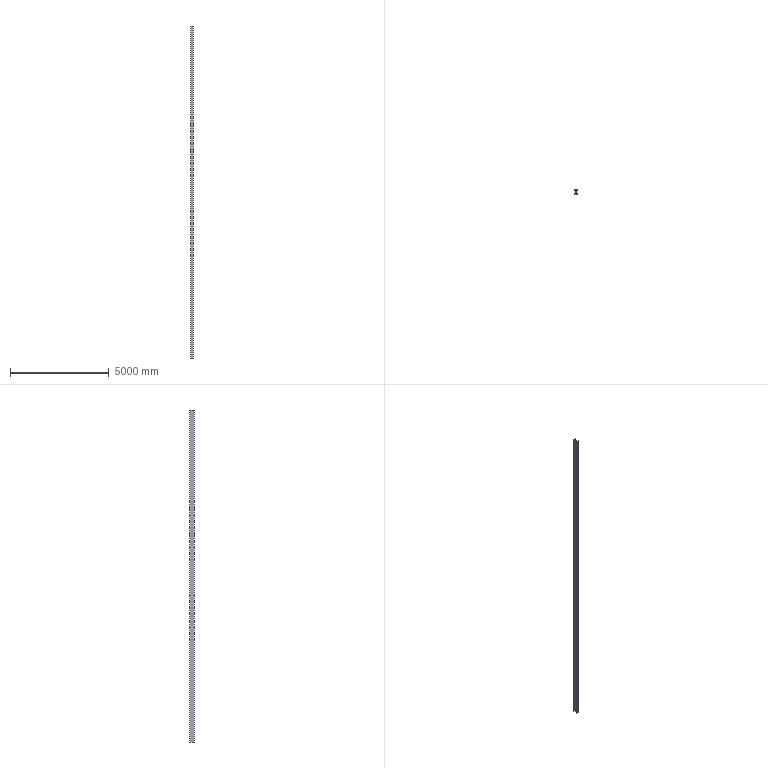Part | SolidWorks | features Extrusion 1 | 1 solid | 18 faces | box 125 x 250 x 16840 mm | volume 62256437 mm3 | plane 14 | cylinder 4 | commonest cylinder face diameters 16 x4
STEP:
#1=CARTESIAN_POINT('',(-62.5,9.,0.));
#2=VERTEX_POINT('',#1);
#3=CARTESIAN_POINT('',(-62.5,0.,0.));
#4=VERTEX_POINT('',#3);
#5=CARTESIAN_POINT('',(-62.5,0.,0.));
#6=DIRECTION('',(0.,-1.,0.));
#7=VECTOR('',#6,1000.);
#8=LINE('',#5,#7);
#9=EDGE_CURVE('',#2,#4,#8,.T.);
#10=ORIENTED_EDGE('',*,*,#9,.T.);
#11=CARTESIAN_POINT('',(-62.5,0.,16840.));
#12=VERTEX_POINT('',#11);
#13=CARTESIAN_POINT('',(-62.5,0.,16840.));
#14=DIRECTION('',(0.,0.,-1.));
#15=VECTOR('',#14,1000.);
#16=LINE('',#13,#15);
#17=EDGE_CURVE('',#12,#4,#16,.T.);
#18=ORIENTED_EDGE('',*,*,#17,.F.);
#19=CARTESIAN_POINT('',(-62.5,9.,16840.));
#20=VERTEX_POINT('',#19);
#21=CARTESIAN_POINT('',(-62.5,0.,16840.));
#22=DIRECTION('',(0.,-1.,0.));
#23=VECTOR('',#22,1000.);
#24=LINE('',#21,#23);
#25=EDGE_CURVE('',#20,#12,#24,.T.);
#26=ORIENTED_EDGE('',*,*,#25,.F.);
#27=CARTESIAN_POINT('',(-62.5,9.,16840.));
#28=DIRECTION('',(0.,0.,-1.));
#29=VECTOR('',#28,1000.);
#30=LINE('',#27,#29);
#31=EDGE_CURVE('',#20,#2,#30,.T.);
#32=ORIENTED_EDGE('',*,*,#31,.T.);
#33=EDGE_LOOP('',(#10,#18,#26,#32));
#34=FACE_OUTER_BOUND('',#33,.T.);
#35=CARTESIAN_POINT('',(-62.5,0.,16840.));
#36=DIRECTION('',(1.,0.,0.));
#37=DIRECTION('',(0.,0.,-1.));
#38=AXIS2_PLACEMENT_3D('',#35,#36,#37);
#39=PLANE('',#38);
#40=ADVANCED_FACE('',(#34),#39,.F.);
#41=CARTESIAN_POINT('',(62.5,0.,0.));
#42=VERTEX_POINT('',#41);
#43=CARTESIAN_POINT('',(62.5,0.,0.));
#44=DIRECTION('',(1.,0.,0.));
#45=VECTOR('',#44,1000.);
#46=LINE('',#43,#45);
#47=EDGE_CURVE('',#4,#42,#46,.T.);
#48=ORIENTED_EDGE('',*,*,#47,.T.);
#49=CARTESIAN_POINT('',(62.5,0.,16840.));
#50=VERTEX_POINT('',#49);
#51=CARTESIAN_POINT('',(62.5,0.,16840.));
#52=DIRECTION('',(0.,0.,-1.));
#53=VECTOR('',#52,1000.);
#54=LINE('',#51,#53);
#55=EDGE_CURVE('',#50,#42,#54,.T.);
#56=ORIENTED_EDGE('',*,*,#55,.F.);
#57=CARTESIAN_POINT('',(62.5,0.,16840.));
#58=DIRECTION('',(1.,0.,0.));
#59=VECTOR('',#58,1000.);
#60=LINE('',#57,#59);
#61=EDGE_CURVE('',#12,#50,#60,.T.);
#62=ORIENTED_EDGE('',*,*,#61,.F.);
#63=ORIENTED_EDGE('',*,*,#17,.T.);
#64=EDGE_LOOP('',(#48,#56,#62,#63));
#65=FACE_OUTER_BOUND('',#64,.T.);
#66=CARTESIAN_POINT('',(62.5,0.,16840.));
#67=DIRECTION('',(0.,1.,0.));
#68=DIRECTION('',(0.,0.,1.));
#69=AXIS2_PLACEMENT_3D('',#66,#67,#68);
#70=PLANE('',#69);
#71=ADVANCED_FACE('',(#65),#70,.F.);
#72=CARTESIAN_POINT('',(62.5,9.,0.));
#73=VERTEX_POINT('',#72);
#74=CARTESIAN_POINT('',(62.5,0.,0.));
#75=DIRECTION('',(0.,1.,0.));
#76=VECTOR('',#75,1000.);
#77=LINE('',#74,#76);
#78=EDGE_CURVE('',#42,#73,#77,.T.);
#79=ORIENTED_EDGE('',*,*,#78,.T.);
#80=CARTESIAN_POINT('',(62.5,9.,16840.));
#81=VERTEX_POINT('',#80);
#82=CARTESIAN_POINT('',(62.5,9.,16840.));
#83=DIRECTION('',(0.,0.,-1.));
#84=VECTOR('',#83,1000.);
#85=LINE('',#82,#84);
#86=EDGE_CURVE('',#81,#73,#85,.T.);
#87=ORIENTED_EDGE('',*,*,#86,.F.);
#88=CARTESIAN_POINT('',(62.5,0.,16840.));
#89=DIRECTION('',(0.,1.,0.));
#90=VECTOR('',#89,1000.);
#91=LINE('',#88,#90);
#92=EDGE_CURVE('',#50,#81,#91,.T.);
#93=ORIENTED_EDGE('',*,*,#92,.F.);
#94=ORIENTED_EDGE('',*,*,#55,.T.);
#95=EDGE_LOOP('',(#79,#87,#93,#94));
#96=FACE_OUTER_BOUND('',#95,.T.);
#97=CARTESIAN_POINT('',(62.5,0.,16840.));
#98=DIRECTION('',(-1.,0.,0.));
#99=DIRECTION('',(0.,0.,1.));
#100=AXIS2_PLACEMENT_3D('',#97,#98,#99);
#101=PLANE('',#100);
#102=ADVANCED_FACE('',(#96),#101,.F.);
#103=CARTESIAN_POINT('',(11.,9.,0.));
#104=VERTEX_POINT('',#103);
#105=CARTESIAN_POINT('',(62.5,9.,0.));
#106=DIRECTION('',(-1.,0.,0.));
#107=VECTOR('',#106,1000.);
#108=LINE('',#105,#107);
#109=EDGE_CURVE('',#73,#104,#108,.T.);
#110=ORIENTED_EDGE('',*,*,#109,.T.);
#111=CARTESIAN_POINT('',(11.,9.,16840.));
#112=VERTEX_POINT('',#111);
#113=CARTESIAN_POINT('',(11.,9.,16840.));
#114=DIRECTION('',(0.,0.,-1.));
#115=VECTOR('',#114,1000.);
#116=LINE('',#113,#115);
#117=EDGE_CURVE('',#112,#104,#116,.T.);
#118=ORIENTED_EDGE('',*,*,#117,.F.);
#119=CARTESIAN_POINT('',(62.5,9.,16840.));
#120=DIRECTION('',(-1.,0.,0.));
#121=VECTOR('',#120,1000.);
#122=LINE('',#119,#121);
#123=EDGE_CURVE('',#81,#112,#122,.T.);
#124=ORIENTED_EDGE('',*,*,#123,.F.);
#125=ORIENTED_EDGE('',*,*,#86,.T.);
#126=EDGE_LOOP('',(#110,#118,#124,#125));
#127=FACE_OUTER_BOUND('',#126,.T.);
#128=CARTESIAN_POINT('',(62.5,9.,16840.));
#129=DIRECTION('',(0.,-1.,0.));
#130=DIRECTION('',(0.,0.,-1.));
#131=AXIS2_PLACEMENT_3D('',#128,#129,#130);
#132=PLANE('',#131);
#133=ADVANCED_FACE('',(#127),#132,.F.);
#134=CARTESIAN_POINT('',(3.,17.,0.));
#135=VERTEX_POINT('',#134);
#136=CARTESIAN_POINT('',(11.,17.,0.));
#137=DIRECTION('',(0.,0.,-1.));
#138=DIRECTION('',(-1.,0.,0.));
#139=AXIS2_PLACEMENT_3D('',#136,#137,#138);
#140=CIRCLE('',#139,8.);
#141=EDGE_CURVE('',#104,#135,#140,.T.);
#142=ORIENTED_EDGE('',*,*,#141,.T.);
#143=CARTESIAN_POINT('',(3.,17.,16840.));
#144=VERTEX_POINT('',#143);
#145=CARTESIAN_POINT('',(3.,17.,16840.));
#146=DIRECTION('',(0.,0.,-1.));
#147=VECTOR('',#146,1000.);
#148=LINE('',#145,#147);
#149=EDGE_CURVE('',#144,#135,#148,.T.);
#150=ORIENTED_EDGE('',*,*,#149,.F.);
#151=CARTESIAN_POINT('',(11.,17.,16840.));
#152=DIRECTION('',(0.,0.,-1.));
#153=DIRECTION('',(-1.,0.,0.));
#154=AXIS2_PLACEMENT_3D('',#151,#152,#153);
#155=CIRCLE('',#154,8.);
#156=EDGE_CURVE('',#112,#144,#155,.T.);
#157=ORIENTED_EDGE('',*,*,#156,.F.);
#158=ORIENTED_EDGE('',*,*,#117,.T.);
#159=EDGE_LOOP('',(#142,#150,#157,#158));
#160=FACE_OUTER_BOUND('',#159,.T.);
#161=CARTESIAN_POINT('',(11.,17.,16840.));
#162=DIRECTION('',(0.,0.,-1.));
#163=DIRECTION('',(-1.,0.,0.));
#164=AXIS2_PLACEMENT_3D('',#161,#162,#163);
#165=CYLINDRICAL_SURFACE('',#164,8.);
#166=ADVANCED_FACE('',(#160),#165,.F.);
#167=CARTESIAN_POINT('',(3.,233.,0.));
#168=VERTEX_POINT('',#167);
#169=CARTESIAN_POINT('',(3.,17.,0.));
#170=DIRECTION('',(0.,1.,0.));
#171=VECTOR('',#170,1000.);
#172=LINE('',#169,#171);
#173=EDGE_CURVE('',#135,#168,#172,.T.);
#174=ORIENTED_EDGE('',*,*,#173,.T.);
#175=CARTESIAN_POINT('',(3.,233.,16840.));
#176=VERTEX_POINT('',#175);
#177=CARTESIAN_POINT('',(3.,233.,16840.));
#178=DIRECTION('',(0.,0.,-1.));
#179=VECTOR('',#178,1000.);
#180=LINE('',#177,#179);
#181=EDGE_CURVE('',#176,#168,#180,.T.);
#182=ORIENTED_EDGE('',*,*,#181,.F.);
#183=CARTESIAN_POINT('',(3.,17.,16840.));
#184=DIRECTION('',(0.,1.,0.));
#185=VECTOR('',#184,1000.);
#186=LINE('',#183,#185);
#187=EDGE_CURVE('',#144,#176,#186,.T.);
#188=ORIENTED_EDGE('',*,*,#187,.F.);
#189=ORIENTED_EDGE('',*,*,#149,.T.);
#190=EDGE_LOOP('',(#174,#182,#188,#189));
#191=FACE_OUTER_BOUND('',#190,.T.);
#192=CARTESIAN_POINT('',(3.,17.,16840.));
#193=DIRECTION('',(-1.,0.,0.));
#194=DIRECTION('',(0.,-1.,0.));
#195=AXIS2_PLACEMENT_3D('',#192,#193,#194);
#196=PLANE('',#195);
#197=ADVANCED_FACE('',(#191),#196,.F.);
#198=CARTESIAN_POINT('',(11.,241.,0.));
#199=VERTEX_POINT('',#198);
#200=CARTESIAN_POINT('',(11.,233.,0.));
#201=DIRECTION('',(0.,0.,-1.));
#202=DIRECTION('',(-1.,0.,0.));
#203=AXIS2_PLACEMENT_3D('',#200,#201,#202);
#204=CIRCLE('',#203,8.);
#205=EDGE_CURVE('',#168,#199,#204,.T.);
#206=ORIENTED_EDGE('',*,*,#205,.T.);
#207=CARTESIAN_POINT('',(11.,241.,16840.));
#208=VERTEX_POINT('',#207);
#209=CARTESIAN_POINT('',(11.,241.,16840.));
#210=DIRECTION('',(0.,0.,-1.));
#211=VECTOR('',#210,1000.);
#212=LINE('',#209,#211);
#213=EDGE_CURVE('',#208,#199,#212,.T.);
#214=ORIENTED_EDGE('',*,*,#213,.F.);
#215=CARTESIAN_POINT('',(11.,233.,16840.));
#216=DIRECTION('',(0.,0.,-1.));
#217=DIRECTION('',(-1.,0.,0.));
#218=AXIS2_PLACEMENT_3D('',#215,#216,#217);
#219=CIRCLE('',#218,8.);
#220=EDGE_CURVE('',#176,#208,#219,.T.);
#221=ORIENTED_EDGE('',*,*,#220,.F.);
#222=ORIENTED_EDGE('',*,*,#181,.T.);
#223=EDGE_LOOP('',(#206,#214,#221,#222));
#224=FACE_OUTER_BOUND('',#223,.T.);
#225=CARTESIAN_POINT('',(11.,233.,16840.));
#226=DIRECTION('',(0.,0.,-1.));
#227=DIRECTION('',(-1.,0.,0.));
#228=AXIS2_PLACEMENT_3D('',#225,#226,#227);
#229=CYLINDRICAL_SURFACE('',#228,8.);
#230=ADVANCED_FACE('',(#224),#229,.F.);
#231=CARTESIAN_POINT('',(62.5,241.,0.));
#232=VERTEX_POINT('',#231);
#233=CARTESIAN_POINT('',(11.,241.,0.));
#234=DIRECTION('',(1.,0.,0.));
#235=VECTOR('',#234,1000.);
#236=LINE('',#233,#235);
#237=EDGE_CURVE('',#199,#232,#236,.T.);
#238=ORIENTED_EDGE('',*,*,#237,.T.);
#239=CARTESIAN_POINT('',(62.5,241.,16840.));
#240=VERTEX_POINT('',#239);
#241=CARTESIAN_POINT('',(62.5,241.,16840.));
#242=DIRECTION('',(0.,0.,-1.));
#243=VECTOR('',#242,1000.);
#244=LINE('',#241,#243);
#245=EDGE_CURVE('',#240,#232,#244,.T.);
#246=ORIENTED_EDGE('',*,*,#245,.F.);
#247=CARTESIAN_POINT('',(11.,241.,16840.));
#248=DIRECTION('',(1.,0.,0.));
#249=VECTOR('',#248,1000.);
#250=LINE('',#247,#249);
#251=EDGE_CURVE('',#208,#240,#250,.T.);
#252=ORIENTED_EDGE('',*,*,#251,.F.);
#253=ORIENTED_EDGE('',*,*,#213,.T.);
#254=EDGE_LOOP('',(#238,#246,#252,#253));
#255=FACE_OUTER_BOUND('',#254,.T.);
#256=CARTESIAN_POINT('',(11.,241.,16840.));
#257=DIRECTION('',(0.,1.,0.));
#258=DIRECTION('',(0.,0.,1.));
#259=AXIS2_PLACEMENT_3D('',#256,#257,#258);
#260=PLANE('',#259);
#261=ADVANCED_FACE('',(#255),#260,.F.);
#262=CARTESIAN_POINT('',(62.5,250.,0.));
#263=VERTEX_POINT('',#262);
#264=CARTESIAN_POINT('',(62.5,241.,0.));
#265=DIRECTION('',(0.,1.,0.));
#266=VECTOR('',#265,1000.);
#267=LINE('',#264,#266);
#268=EDGE_CURVE('',#232,#263,#267,.T.);
#269=ORIENTED_EDGE('',*,*,#268,.T.);
#270=CARTESIAN_POINT('',(62.5,250.,16840.));
#271=VERTEX_POINT('',#270);
#272=CARTESIAN_POINT('',(62.5,250.,16840.));
#273=DIRECTION('',(0.,0.,-1.));
#274=VECTOR('',#273,1000.);
#275=LINE('',#272,#274);
#276=EDGE_CURVE('',#271,#263,#275,.T.);
#277=ORIENTED_EDGE('',*,*,#276,.F.);
#278=CARTESIAN_POINT('',(62.5,241.,16840.));
#279=DIRECTION('',(0.,1.,0.));
#280=VECTOR('',#279,1000.);
#281=LINE('',#278,#280);
#282=EDGE_CURVE('',#240,#271,#281,.T.);
#283=ORIENTED_EDGE('',*,*,#282,.F.);
#284=ORIENTED_EDGE('',*,*,#245,.T.);
#285=EDGE_LOOP('',(#269,#277,#283,#284));
#286=FACE_OUTER_BOUND('',#285,.T.);
#287=CARTESIAN_POINT('',(62.5,241.,16840.));
#288=DIRECTION('',(-1.,0.,0.));
#289=DIRECTION('',(0.,0.,1.));
#290=AXIS2_PLACEMENT_3D('',#287,#288,#289);
#291=PLANE('',#290);
#292=ADVANCED_FACE('',(#286),#291,.F.);
#293=CARTESIAN_POINT('',(-62.5,250.,0.));
#294=VERTEX_POINT('',#293);
#295=CARTESIAN_POINT('',(-62.5,250.,0.));
#296=DIRECTION('',(-1.,0.,0.));
#297=VECTOR('',#296,1000.);
#298=LINE('',#295,#297);
#299=EDGE_CURVE('',#263,#294,#298,.T.);
#300=ORIENTED_EDGE('',*,*,#299,.T.);
#301=CARTESIAN_POINT('',(-62.5,250.,16840.));
#302=VERTEX_POINT('',#301);
#303=CARTESIAN_POINT('',(-62.5,250.,16840.));
#304=DIRECTION('',(0.,0.,-1.));
#305=VECTOR('',#304,1000.);
#306=LINE('',#303,#305);
#307=EDGE_CURVE('',#302,#294,#306,.T.);
#308=ORIENTED_EDGE('',*,*,#307,.F.);
#309=CARTESIAN_POINT('',(-62.5,250.,16840.));
#310=DIRECTION('',(-1.,0.,0.));
#311=VECTOR('',#310,1000.);
#312=LINE('',#309,#311);
#313=EDGE_CURVE('',#271,#302,#312,.T.);
#314=ORIENTED_EDGE('',*,*,#313,.F.);
#315=ORIENTED_EDGE('',*,*,#276,.T.);
#316=EDGE_LOOP('',(#300,#308,#314,#315));
#317=FACE_OUTER_BOUND('',#316,.T.);
#318=CARTESIAN_POINT('',(-62.5,250.,16840.));
#319=DIRECTION('',(0.,-1.,0.));
#320=DIRECTION('',(1.,0.,0.));
#321=AXIS2_PLACEMENT_3D('',#318,#319,#320);
#322=PLANE('',#321);
#323=ADVANCED_FACE('',(#317),#322,.F.);
#324=CARTESIAN_POINT('',(-62.5,241.,0.));
#325=VERTEX_POINT('',#324);
#326=CARTESIAN_POINT('',(-62.5,241.,0.));
#327=DIRECTION('',(0.,-1.,0.));
#328=VECTOR('',#327,1000.);
#329=LINE('',#326,#328);
#330=EDGE_CURVE('',#294,#325,#329,.T.);
#331=ORIENTED_EDGE('',*,*,#330,.T.);
#332=CARTESIAN_POINT('',(-62.5,241.,16840.));
#333=VERTEX_POINT('',#332);
#334=CARTESIAN_POINT('',(-62.5,241.,16840.));
#335=DIRECTION('',(0.,0.,-1.));
#336=VECTOR('',#335,1000.);
#337=LINE('',#334,#336);
#338=EDGE_CURVE('',#333,#325,#337,.T.);
#339=ORIENTED_EDGE('',*,*,#338,.F.);
#340=CARTESIAN_POINT('',(-62.5,241.,16840.));
#341=DIRECTION('',(0.,-1.,0.));
#342=VECTOR('',#341,1000.);
#343=LINE('',#340,#342);
#344=EDGE_CURVE('',#302,#333,#343,.T.);
#345=ORIENTED_EDGE('',*,*,#344,.F.);
#346=ORIENTED_EDGE('',*,*,#307,.T.);
#347=EDGE_LOOP('',(#331,#339,#345,#346));
#348=FACE_OUTER_BOUND('',#347,.T.);
#349=CARTESIAN_POINT('',(-62.5,241.,16840.));
#350=DIRECTION('',(1.,0.,0.));
#351=DIRECTION('',(0.,0.,-1.));
#352=AXIS2_PLACEMENT_3D('',#349,#350,#351);
#353=PLANE('',#352);
#354=ADVANCED_FACE('',(#348),#353,.F.);
#355=CARTESIAN_POINT('',(-11.,241.,0.));
#356=VERTEX_POINT('',#355);
#357=CARTESIAN_POINT('',(-11.,241.,0.));
#358=DIRECTION('',(1.,0.,0.));
#359=VECTOR('',#358,1000.);
#360=LINE('',#357,#359);
#361=EDGE_CURVE('',#325,#356,#360,.T.);
#362=ORIENTED_EDGE('',*,*,#361,.T.);
#363=CARTESIAN_POINT('',(-11.,241.,16840.));
#364=VERTEX_POINT('',#363);
#365=CARTESIAN_POINT('',(-11.,241.,16840.));
#366=DIRECTION('',(0.,0.,-1.));
#367=VECTOR('',#366,1000.);
#368=LINE('',#365,#367);
#369=EDGE_CURVE('',#364,#356,#368,.T.);
#370=ORIENTED_EDGE('',*,*,#369,.F.);
#371=CARTESIAN_POINT('',(-11.,241.,16840.));
#372=DIRECTION('',(1.,0.,0.));
#373=VECTOR('',#372,1000.);
#374=LINE('',#371,#373);
#375=EDGE_CURVE('',#333,#364,#374,.T.);
#376=ORIENTED_EDGE('',*,*,#375,.F.);
#377=ORIENTED_EDGE('',*,*,#338,.T.);
#378=EDGE_LOOP('',(#362,#370,#376,#377));
#379=FACE_OUTER_BOUND('',#378,.T.);
#380=CARTESIAN_POINT('',(-11.,241.,16840.));
#381=DIRECTION('',(0.,1.,0.));
#382=DIRECTION('',(0.,0.,1.));
#383=AXIS2_PLACEMENT_3D('',#380,#381,#382);
#384=PLANE('',#383);
#385=ADVANCED_FACE('',(#379),#384,.F.);
#386=CARTESIAN_POINT('',(-3.,233.,0.));
#387=VERTEX_POINT('',#386);
#388=CARTESIAN_POINT('',(-11.,233.,0.));
#389=DIRECTION('',(0.,0.,-1.));
#390=DIRECTION('',(1.,0.,0.));
#391=AXIS2_PLACEMENT_3D('',#388,#389,#390);
#392=CIRCLE('',#391,8.);
#393=EDGE_CURVE('',#356,#387,#392,.T.);
#394=ORIENTED_EDGE('',*,*,#393,.T.);
#395=CARTESIAN_POINT('',(-3.,233.,16840.));
#396=VERTEX_POINT('',#395);
#397=CARTESIAN_POINT('',(-3.,233.,16840.));
#398=DIRECTION('',(0.,0.,-1.));
#399=VECTOR('',#398,1000.);
#400=LINE('',#397,#399);
#401=EDGE_CURVE('',#396,#387,#400,.T.);
#402=ORIENTED_EDGE('',*,*,#401,.F.);
#403=CARTESIAN_POINT('',(-11.,233.,16840.));
#404=DIRECTION('',(0.,0.,-1.));
#405=DIRECTION('',(1.,0.,0.));
#406=AXIS2_PLACEMENT_3D('',#403,#404,#405);
#407=CIRCLE('',#406,8.);
#408=EDGE_CURVE('',#364,#396,#407,.T.);
#409=ORIENTED_EDGE('',*,*,#408,.F.);
#410=ORIENTED_EDGE('',*,*,#369,.T.);
#411=EDGE_LOOP('',(#394,#402,#409,#410));
#412=FACE_OUTER_BOUND('',#411,.T.);
#413=CARTESIAN_POINT('',(-11.,233.,16840.));
#414=DIRECTION('',(0.,0.,-1.));
#415=DIRECTION('',(-1.,0.,0.));
#416=AXIS2_PLACEMENT_3D('',#413,#414,#415);
#417=CYLINDRICAL_SURFACE('',#416,8.);
#418=ADVANCED_FACE('',(#412),#417,.F.);
#419=CARTESIAN_POINT('',(-3.,17.,0.));
#420=VERTEX_POINT('',#419);
#421=CARTESIAN_POINT('',(-3.,17.,0.));
#422=DIRECTION('',(0.,-1.,0.));
#423=VECTOR('',#422,1000.);
#424=LINE('',#421,#423);
#425=EDGE_CURVE('',#387,#420,#424,.T.);
#426=ORIENTED_EDGE('',*,*,#425,.T.);
#427=CARTESIAN_POINT('',(-3.,17.,16840.));
#428=VERTEX_POINT('',#427);
#429=CARTESIAN_POINT('',(-3.,17.,16840.));
#430=DIRECTION('',(0.,0.,-1.));
#431=VECTOR('',#430,1000.);
#432=LINE('',#429,#431);
#433=EDGE_CURVE('',#428,#420,#432,.T.);
#434=ORIENTED_EDGE('',*,*,#433,.F.);
#435=CARTESIAN_POINT('',(-3.,17.,16840.));
#436=DIRECTION('',(0.,-1.,0.));
#437=VECTOR('',#436,1000.);
#438=LINE('',#435,#437);
#439=EDGE_CURVE('',#396,#428,#438,.T.);
#440=ORIENTED_EDGE('',*,*,#439,.F.);
#441=ORIENTED_EDGE('',*,*,#401,.T.);
#442=EDGE_LOOP('',(#426,#434,#440,#441));
#443=FACE_OUTER_BOUND('',#442,.T.);
#444=CARTESIAN_POINT('',(-3.,17.,16840.));
#445=DIRECTION('',(1.,0.,0.));
#446=DIRECTION('',(0.,1.,0.));
#447=AXIS2_PLACEMENT_3D('',#444,#445,#446);
#448=PLANE('',#447);
#449=ADVANCED_FACE('',(#443),#448,.F.);
#450=CARTESIAN_POINT('',(-11.,9.,0.));
#451=VERTEX_POINT('',#450);
#452=CARTESIAN_POINT('',(-11.,17.,0.));
#453=DIRECTION('',(0.,0.,-1.));
#454=DIRECTION('',(-1.,0.,0.));
#455=AXIS2_PLACEMENT_3D('',#452,#453,#454);
#456=CIRCLE('',#455,8.);
#457=EDGE_CURVE('',#420,#451,#456,.T.);
#458=ORIENTED_EDGE('',*,*,#457,.T.);
#459=CARTESIAN_POINT('',(-11.,9.,16840.));
#460=VERTEX_POINT('',#459);
#461=CARTESIAN_POINT('',(-11.,9.,16840.));
#462=DIRECTION('',(0.,0.,-1.));
#463=VECTOR('',#462,1000.);
#464=LINE('',#461,#463);
#465=EDGE_CURVE('',#460,#451,#464,.T.);
#466=ORIENTED_EDGE('',*,*,#465,.F.);
#467=CARTESIAN_POINT('',(-11.,17.,16840.));
#468=DIRECTION('',(0.,0.,-1.));
#469=DIRECTION('',(-1.,0.,0.));
#470=AXIS2_PLACEMENT_3D('',#467,#468,#469);
#471=CIRCLE('',#470,8.);
#472=EDGE_CURVE('',#428,#460,#471,.T.);
#473=ORIENTED_EDGE('',*,*,#472,.F.);
#474=ORIENTED_EDGE('',*,*,#433,.T.);
#475=EDGE_LOOP('',(#458,#466,#473,#474));
#476=FACE_OUTER_BOUND('',#475,.T.);
#477=CARTESIAN_POINT('',(-11.,17.,16840.));
#478=DIRECTION('',(0.,0.,-1.));
#479=DIRECTION('',(-1.,0.,0.));
#480=AXIS2_PLACEMENT_3D('',#477,#478,#479);
#481=CYLINDRICAL_SURFACE('',#480,8.);
#482=ADVANCED_FACE('',(#476),#481,.F.);
#483=CARTESIAN_POINT('',(-62.5,9.,0.));
#484=DIRECTION('',(-1.,0.,0.));
#485=VECTOR('',#484,1000.);
#486=LINE('',#483,#485);
#487=EDGE_CURVE('',#451,#2,#486,.T.);
#488=ORIENTED_EDGE('',*,*,#487,.T.);
#489=ORIENTED_EDGE('',*,*,#31,.F.);
#490=CARTESIAN_POINT('',(-62.5,9.,16840.));
#491=DIRECTION('',(-1.,0.,0.));
#492=VECTOR('',#491,1000.);
#493=LINE('',#490,#492);
#494=EDGE_CURVE('',#460,#20,#493,.T.);
#495=ORIENTED_EDGE('',*,*,#494,.F.);
#496=ORIENTED_EDGE('',*,*,#465,.T.);
#497=EDGE_LOOP('',(#488,#489,#495,#496));
#498=FACE_OUTER_BOUND('',#497,.T.);
#499=CARTESIAN_POINT('',(-62.5,9.,16840.));
#500=DIRECTION('',(0.,-1.,0.));
#501=DIRECTION('',(0.,0.,-1.));
#502=AXIS2_PLACEMENT_3D('',#499,#500,#501);
#503=PLANE('',#502);
#504=ADVANCED_FACE('',(#498),#503,.F.);
#505=ORIENTED_EDGE('',*,*,#25,.T.);
#506=ORIENTED_EDGE('',*,*,#61,.T.);
#507=ORIENTED_EDGE('',*,*,#92,.T.);
#508=ORIENTED_EDGE('',*,*,#123,.T.);
#509=ORIENTED_EDGE('',*,*,#156,.T.);
#510=ORIENTED_EDGE('',*,*,#187,.T.);
#511=ORIENTED_EDGE('',*,*,#220,.T.);
#512=ORIENTED_EDGE('',*,*,#251,.T.);
#513=ORIENTED_EDGE('',*,*,#282,.T.);
#514=ORIENTED_EDGE('',*,*,#313,.T.);
#515=ORIENTED_EDGE('',*,*,#344,.T.);
#516=ORIENTED_EDGE('',*,*,#375,.T.);
#517=ORIENTED_EDGE('',*,*,#408,.T.);
#518=ORIENTED_EDGE('',*,*,#439,.T.);
#519=ORIENTED_EDGE('',*,*,#472,.T.);
#520=ORIENTED_EDGE('',*,*,#494,.T.);
#521=EDGE_LOOP('',(#505,#506,#507,#508,#509,#510,#511,#512,#513,#514,#515,#516,#517,#518,#519,#520));
#522=FACE_OUTER_BOUND('',#521,.T.);
#523=CARTESIAN_POINT('',(-11.,17.,16840.));
#524=DIRECTION('',(0.,0.,-1.));
#525=DIRECTION('',(-1.,0.,0.));
#526=AXIS2_PLACEMENT_3D('',#523,#524,#525);
#527=PLANE('',#526);
#528=ADVANCED_FACE('',(#522),#527,.F.);
#529=ORIENTED_EDGE('',*,*,#9,.F.);
#530=ORIENTED_EDGE('',*,*,#487,.F.);
#531=ORIENTED_EDGE('',*,*,#457,.F.);
#532=ORIENTED_EDGE('',*,*,#425,.F.);
#533=ORIENTED_EDGE('',*,*,#393,.F.);
#534=ORIENTED_EDGE('',*,*,#361,.F.);
#535=ORIENTED_EDGE('',*,*,#330,.F.);
#536=ORIENTED_EDGE('',*,*,#299,.F.);
#537=ORIENTED_EDGE('',*,*,#268,.F.);
#538=ORIENTED_EDGE('',*,*,#237,.F.);
#539=ORIENTED_EDGE('',*,*,#205,.F.);
#540=ORIENTED_EDGE('',*,*,#173,.F.);
#541=ORIENTED_EDGE('',*,*,#141,.F.);
#542=ORIENTED_EDGE('',*,*,#109,.F.);
#543=ORIENTED_EDGE('',*,*,#78,.F.);
#544=ORIENTED_EDGE('',*,*,#47,.F.);
#545=EDGE_LOOP('',(#529,#530,#531,#532,#533,#534,#535,#536,#537,#538,#539,#540,#541,#542,#543,#544));
#546=FACE_OUTER_BOUND('',#545,.T.);
#547=CARTESIAN_POINT('',(-11.,17.,0.));
#548=DIRECTION('',(0.,0.,-1.));
#549=DIRECTION('',(-1.,0.,0.));
#550=AXIS2_PLACEMENT_3D('',#547,#548,#549);
#551=PLANE('',#550);
#552=ADVANCED_FACE('',(#546),#551,.T.);
#553=CLOSED_SHELL('',(#40,#71,#102,#133,#166,#197,#230,#261,#292,#323,#354,#385,#418,#449,#482,#504,#528,#552));
#554=MANIFOLD_SOLID_BREP('',#553);
#555=CARTESIAN_POINT('',(0.,0.,0.));
#556=DIRECTION('',(0.,0.,1.));
#557=DIRECTION('',(1.,0.,0.));
#558=AXIS2_PLACEMENT_3D('',#555,#556,#557);
#559=(LENGTH_UNIT()NAMED_UNIT(*)SI_UNIT(.MILLI.,.METRE.));
#560=UNCERTAINTY_MEASURE_WITH_UNIT(LENGTH_MEASURE(0.00001),#559,'','');
#561=(NAMED_UNIT(*)PLANE_ANGLE_UNIT()SI_UNIT($,.RADIAN.));
#562=(NAMED_UNIT(*)SI_UNIT($,.STERADIAN.)SOLID_ANGLE_UNIT());
#563=(GEOMETRIC_REPRESENTATION_CONTEXT(3)GLOBAL_UNCERTAINTY_ASSIGNED_CONTEXT((#560))GLOBAL_UNIT_ASSIGNED_CONTEXT((#559,#561,#562))REPRESENTATION_CONTEXT('',''));
#564=ADVANCED_BREP_SHAPE_REPRESENTATION('',(#554,#558),#563);